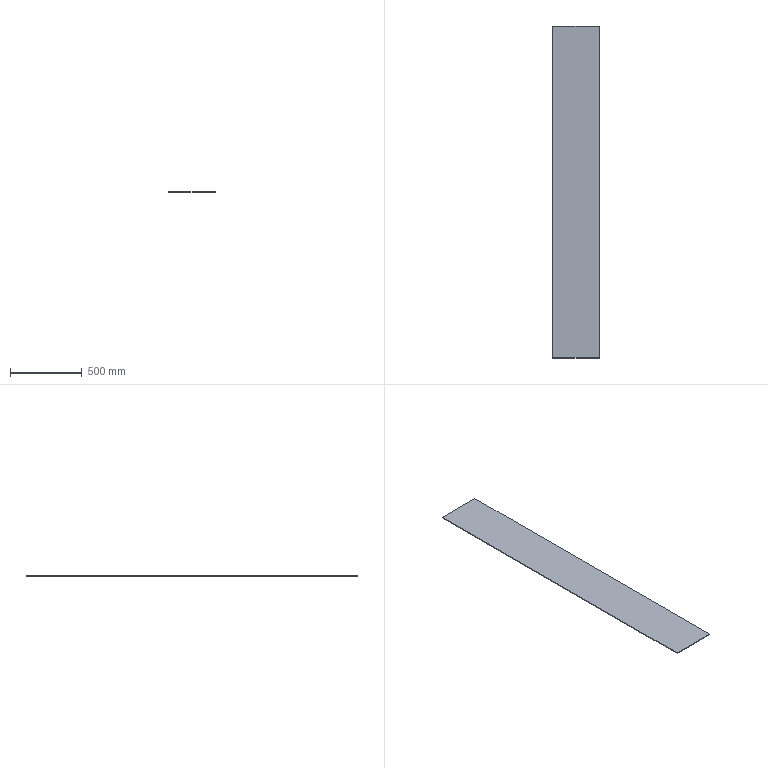Part | SolidWorks | features Extrusion 1, HoleWzd 1 | 1 solid | 6 faces | box 321 x 2310 x 5 mm | volume 3707550 mm3 | plane 6
STEP:
#1=CARTESIAN_POINT('',(160.5,-1155.,0.));
#2=VERTEX_POINT('',#1);
#3=CARTESIAN_POINT('',(160.5,1155.,0.));
#4=VERTEX_POINT('',#3);
#5=CARTESIAN_POINT('',(160.5,1155.,0.));
#6=DIRECTION('',(0.,1.,0.));
#7=VECTOR('',#6,1000.);
#8=LINE('',#5,#7);
#9=EDGE_CURVE('',#2,#4,#8,.T.);
#10=ORIENTED_EDGE('',*,*,#9,.T.);
#11=CARTESIAN_POINT('',(160.5,1155.,5.));
#12=VERTEX_POINT('',#11);
#13=CARTESIAN_POINT('',(160.5,1155.,5.));
#14=DIRECTION('',(0.,0.,-1.));
#15=VECTOR('',#14,1000.);
#16=LINE('',#13,#15);
#17=EDGE_CURVE('',#12,#4,#16,.T.);
#18=ORIENTED_EDGE('',*,*,#17,.F.);
#19=CARTESIAN_POINT('',(160.5,-1155.,5.));
#20=VERTEX_POINT('',#19);
#21=CARTESIAN_POINT('',(160.5,1155.,5.));
#22=DIRECTION('',(0.,1.,0.));
#23=VECTOR('',#22,1000.);
#24=LINE('',#21,#23);
#25=EDGE_CURVE('',#20,#12,#24,.T.);
#26=ORIENTED_EDGE('',*,*,#25,.F.);
#27=CARTESIAN_POINT('',(160.5,-1155.,5.));
#28=DIRECTION('',(0.,0.,-1.));
#29=VECTOR('',#28,1000.);
#30=LINE('',#27,#29);
#31=EDGE_CURVE('',#20,#2,#30,.T.);
#32=ORIENTED_EDGE('',*,*,#31,.T.);
#33=EDGE_LOOP('',(#10,#18,#26,#32));
#34=FACE_OUTER_BOUND('',#33,.T.);
#35=CARTESIAN_POINT('',(160.5,1155.,5.));
#36=DIRECTION('',(-1.,0.,0.));
#37=DIRECTION('',(0.,-1.,0.));
#38=AXIS2_PLACEMENT_3D('',#35,#36,#37);
#39=PLANE('',#38);
#40=ADVANCED_FACE('',(#34),#39,.F.);
#41=CARTESIAN_POINT('',(-160.5,1155.,0.));
#42=VERTEX_POINT('',#41);
#43=CARTESIAN_POINT('',(-160.5,1155.,0.));
#44=DIRECTION('',(-1.,0.,0.));
#45=VECTOR('',#44,1000.);
#46=LINE('',#43,#45);
#47=EDGE_CURVE('',#4,#42,#46,.T.);
#48=ORIENTED_EDGE('',*,*,#47,.T.);
#49=CARTESIAN_POINT('',(-160.5,1155.,5.));
#50=VERTEX_POINT('',#49);
#51=CARTESIAN_POINT('',(-160.5,1155.,5.));
#52=DIRECTION('',(0.,0.,-1.));
#53=VECTOR('',#52,1000.);
#54=LINE('',#51,#53);
#55=EDGE_CURVE('',#50,#42,#54,.T.);
#56=ORIENTED_EDGE('',*,*,#55,.F.);
#57=CARTESIAN_POINT('',(-160.5,1155.,5.));
#58=DIRECTION('',(-1.,0.,0.));
#59=VECTOR('',#58,1000.);
#60=LINE('',#57,#59);
#61=EDGE_CURVE('',#12,#50,#60,.T.);
#62=ORIENTED_EDGE('',*,*,#61,.F.);
#63=ORIENTED_EDGE('',*,*,#17,.T.);
#64=EDGE_LOOP('',(#48,#56,#62,#63));
#65=FACE_OUTER_BOUND('',#64,.T.);
#66=CARTESIAN_POINT('',(-160.5,1155.,5.));
#67=DIRECTION('',(0.,-1.,0.));
#68=DIRECTION('',(0.,0.,-1.));
#69=AXIS2_PLACEMENT_3D('',#66,#67,#68);
#70=PLANE('',#69);
#71=ADVANCED_FACE('',(#65),#70,.F.);
#72=CARTESIAN_POINT('',(-160.5,-1155.,0.));
#73=VERTEX_POINT('',#72);
#74=CARTESIAN_POINT('',(-160.5,1155.,0.));
#75=DIRECTION('',(0.,-1.,0.));
#76=VECTOR('',#75,1000.);
#77=LINE('',#74,#76);
#78=EDGE_CURVE('',#42,#73,#77,.T.);
#79=ORIENTED_EDGE('',*,*,#78,.T.);
#80=CARTESIAN_POINT('',(-160.5,-1155.,5.));
#81=VERTEX_POINT('',#80);
#82=CARTESIAN_POINT('',(-160.5,-1155.,5.));
#83=DIRECTION('',(0.,0.,-1.));
#84=VECTOR('',#83,1000.);
#85=LINE('',#82,#84);
#86=EDGE_CURVE('',#81,#73,#85,.T.);
#87=ORIENTED_EDGE('',*,*,#86,.F.);
#88=CARTESIAN_POINT('',(-160.5,1155.,5.));
#89=DIRECTION('',(0.,-1.,0.));
#90=VECTOR('',#89,1000.);
#91=LINE('',#88,#90);
#92=EDGE_CURVE('',#50,#81,#91,.T.);
#93=ORIENTED_EDGE('',*,*,#92,.F.);
#94=ORIENTED_EDGE('',*,*,#55,.T.);
#95=EDGE_LOOP('',(#79,#87,#93,#94));
#96=FACE_OUTER_BOUND('',#95,.T.);
#97=CARTESIAN_POINT('',(-160.5,1155.,5.));
#98=DIRECTION('',(1.,0.,0.));
#99=DIRECTION('',(0.,1.,0.));
#100=AXIS2_PLACEMENT_3D('',#97,#98,#99);
#101=PLANE('',#100);
#102=ADVANCED_FACE('',(#96),#101,.F.);
#103=CARTESIAN_POINT('',(-160.5,-1155.,0.));
#104=DIRECTION('',(1.,0.,0.));
#105=VECTOR('',#104,1000.);
#106=LINE('',#103,#105);
#107=EDGE_CURVE('',#73,#2,#106,.T.);
#108=ORIENTED_EDGE('',*,*,#107,.T.);
#109=ORIENTED_EDGE('',*,*,#31,.F.);
#110=CARTESIAN_POINT('',(-160.5,-1155.,5.));
#111=DIRECTION('',(1.,0.,0.));
#112=VECTOR('',#111,1000.);
#113=LINE('',#110,#112);
#114=EDGE_CURVE('',#81,#20,#113,.T.);
#115=ORIENTED_EDGE('',*,*,#114,.F.);
#116=ORIENTED_EDGE('',*,*,#86,.T.);
#117=EDGE_LOOP('',(#108,#109,#115,#116));
#118=FACE_OUTER_BOUND('',#117,.T.);
#119=CARTESIAN_POINT('',(-160.5,-1155.,5.));
#120=DIRECTION('',(0.,1.,0.));
#121=DIRECTION('',(0.,0.,1.));
#122=AXIS2_PLACEMENT_3D('',#119,#120,#121);
#123=PLANE('',#122);
#124=ADVANCED_FACE('',(#118),#123,.F.);
#125=ORIENTED_EDGE('',*,*,#25,.T.);
#126=ORIENTED_EDGE('',*,*,#61,.T.);
#127=ORIENTED_EDGE('',*,*,#92,.T.);
#128=ORIENTED_EDGE('',*,*,#114,.T.);
#129=EDGE_LOOP('',(#125,#126,#127,#128));
#130=FACE_OUTER_BOUND('',#129,.T.);
#131=CARTESIAN_POINT('',(0.,0.,5.));
#132=DIRECTION('',(0.,0.,1.));
#133=DIRECTION('',(1.,0.,0.));
#134=AXIS2_PLACEMENT_3D('',#131,#132,#133);
#135=PLANE('',#134);
#136=ADVANCED_FACE('',(#130),#135,.T.);
#137=ORIENTED_EDGE('',*,*,#9,.F.);
#138=ORIENTED_EDGE('',*,*,#107,.F.);
#139=ORIENTED_EDGE('',*,*,#78,.F.);
#140=ORIENTED_EDGE('',*,*,#47,.F.);
#141=EDGE_LOOP('',(#137,#138,#139,#140));
#142=FACE_OUTER_BOUND('',#141,.T.);
#143=CARTESIAN_POINT('',(0.,0.,0.));
#144=DIRECTION('',(0.,0.,1.));
#145=DIRECTION('',(1.,0.,0.));
#146=AXIS2_PLACEMENT_3D('',#143,#144,#145);
#147=PLANE('',#146);
#148=ADVANCED_FACE('',(#142),#147,.F.);
#149=CLOSED_SHELL('',(#40,#71,#102,#124,#136,#148));
#150=MANIFOLD_SOLID_BREP('',#149);
#151=CARTESIAN_POINT('',(0.,0.,0.));
#152=DIRECTION('',(0.,0.,1.));
#153=DIRECTION('',(1.,0.,0.));
#154=AXIS2_PLACEMENT_3D('',#151,#152,#153);
#155=(LENGTH_UNIT()NAMED_UNIT(*)SI_UNIT(.MILLI.,.METRE.));
#156=UNCERTAINTY_MEASURE_WITH_UNIT(LENGTH_MEASURE(0.00001),#155,'','');
#157=(NAMED_UNIT(*)PLANE_ANGLE_UNIT()SI_UNIT($,.RADIAN.));
#158=(NAMED_UNIT(*)SI_UNIT($,.STERADIAN.)SOLID_ANGLE_UNIT());
#159=(GEOMETRIC_REPRESENTATION_CONTEXT(3)GLOBAL_UNCERTAINTY_ASSIGNED_CONTEXT((#156))GLOBAL_UNIT_ASSIGNED_CONTEXT((#155,#157,#158))REPRESENTATION_CONTEXT('',''));
#160=ADVANCED_BREP_SHAPE_REPRESENTATION('',(#150,#154),#159);